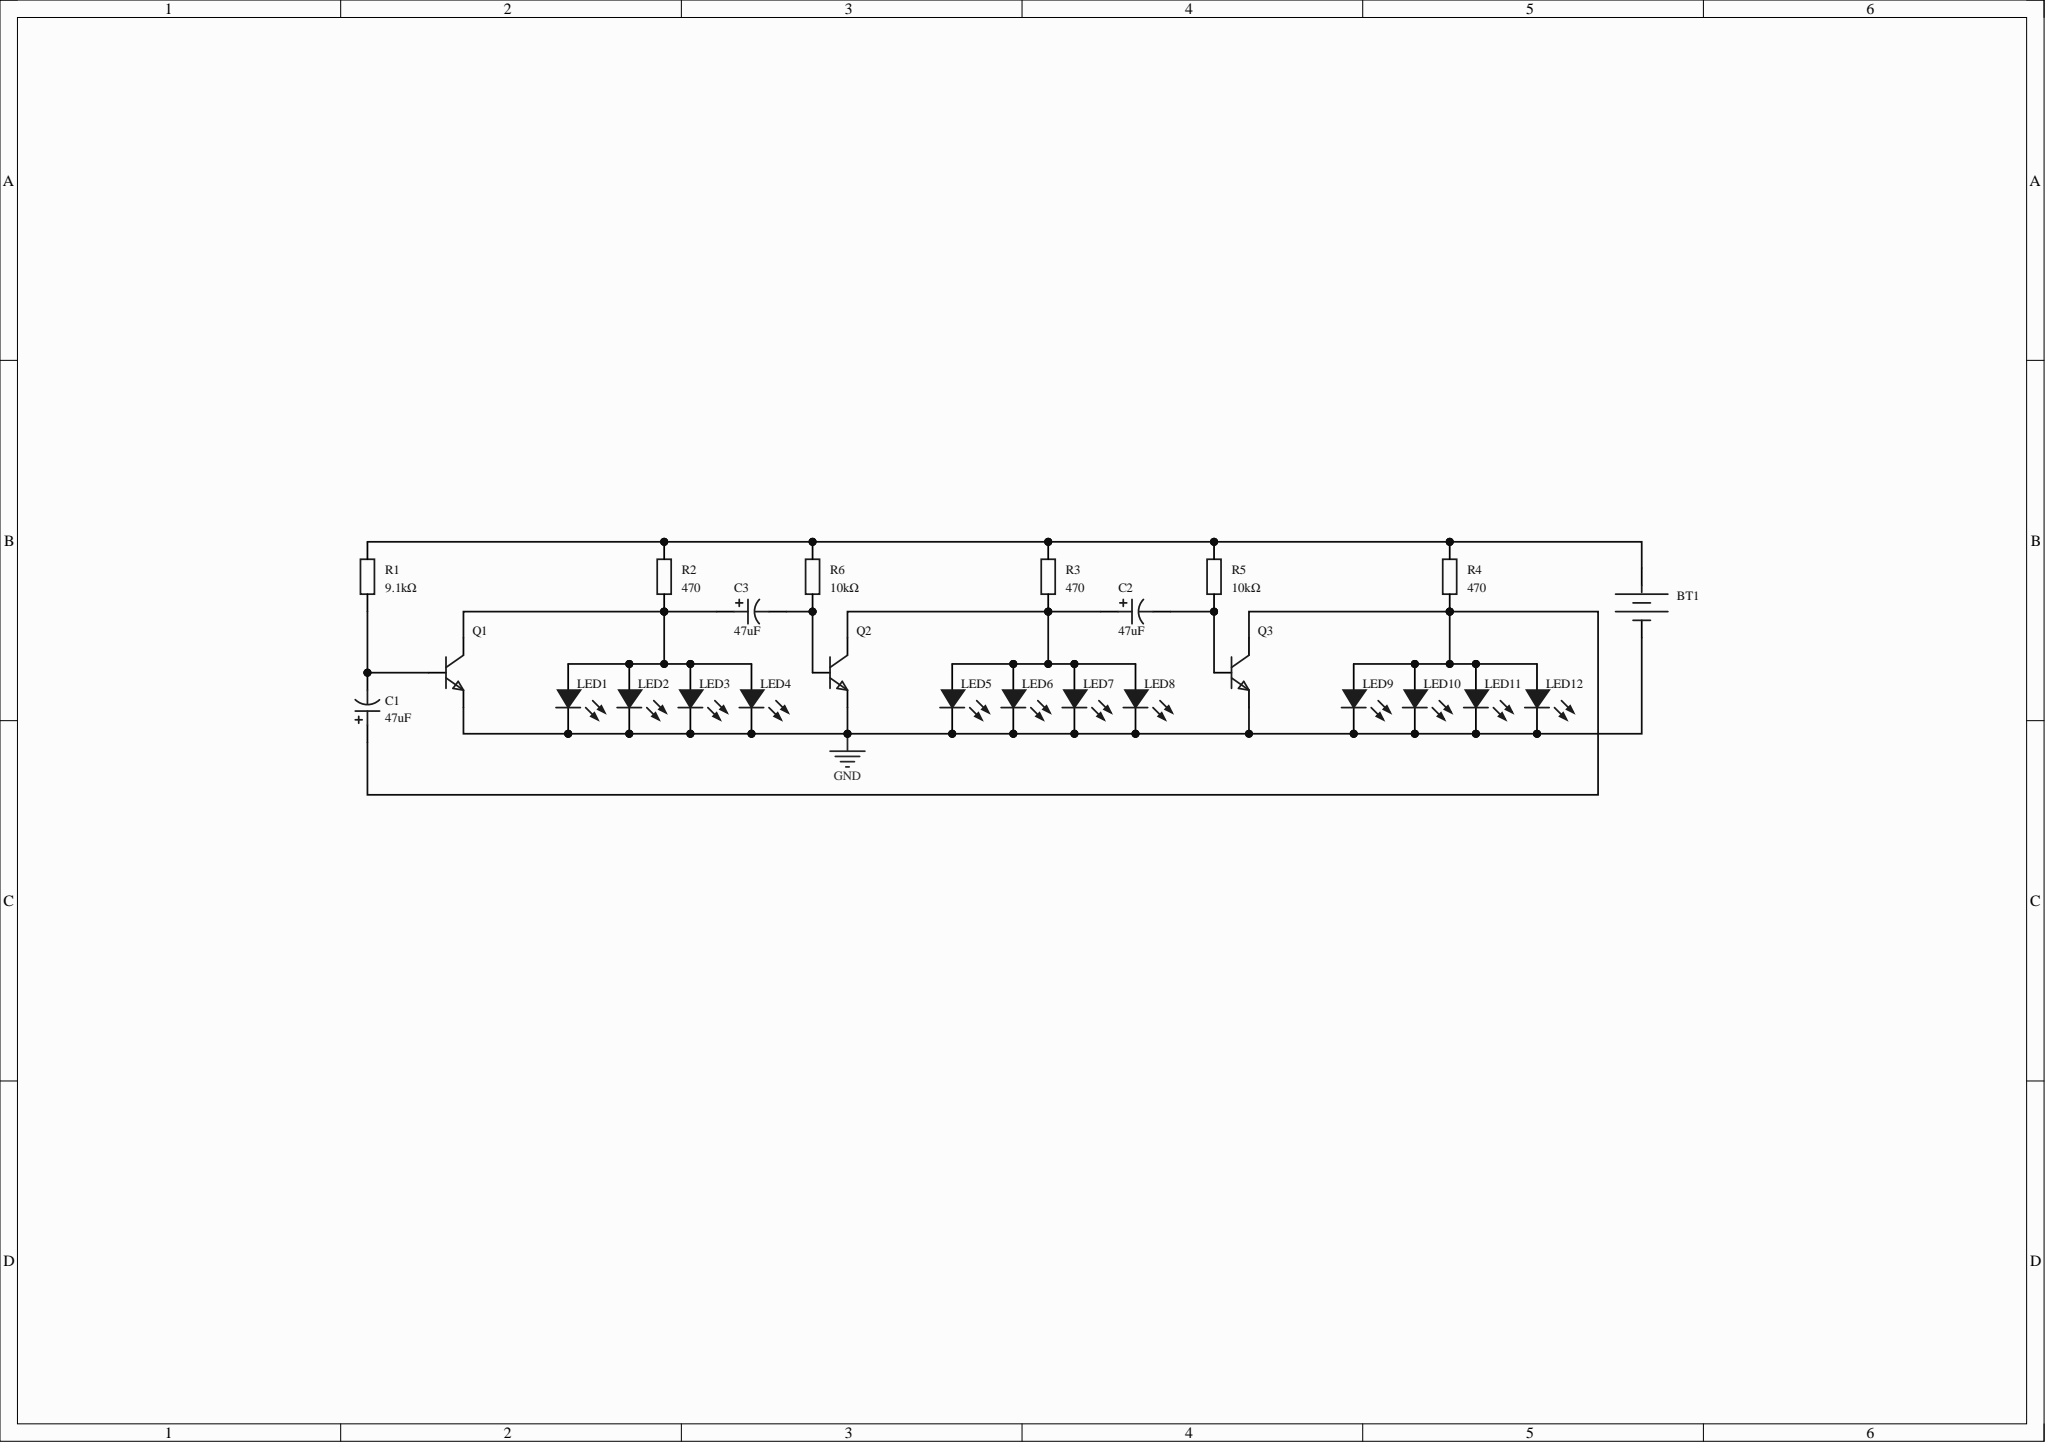Circuit board | Altium Designer | 25 parts | 8 nets
Bill of materials:
Comment,Description,Designator,Footprint,LibRef,Quantity
"9V battery wire clip Cu 100mm","","BT1","BAT-TH_2P-9VBATTERY","9V电池铜线扣 铜100mm","1"
"47uF","","C1, C2, C3","CAP-TH_BD6.3-P2.50-D0.5-FD","DHG016M476E110S1AA","3"
"","","LED1, LED2, LED3, LED4, LED5, LED6, LED7, LED8, LED9, LED10, LED11, LED12","LED-TH_5mm","LED_TH-B_5mm","12"
"","","Q1, Q2, Q3","S8050_TO_92","S8050_TO_NPN","3"
"9.1kΩ","","R1","Res_1/8W","Res_AXIAL-1/8W","1"
"470","","R2, R3, R4","Res_1/8W","Res_AXIAL-1/8W","3"
"10kΩ","","R5, R6","Res_1/8W","Res_AXIAL-1/8W","2"
Netlist (Protel format):
[
BT1
BAT-TH_2P-9VBATTERY
9V battery wire clip Cu 100mm



]
[
C1
CAP-TH_BD6.3-P2.50-D0.5-FD
47uF



]
[
C2
CAP-TH_BD6.3-P2.50-D0.5-FD
47uF



]
[
C3
CAP-TH_BD6.3-P2.50-D0.5-FD
47uF



]
[
LED1
LED-TH_5mm




]
[
LED2
LED-TH_5mm




]
[
LED3
LED-TH_5mm




]
[
LED4
LED-TH_5mm




]
[
LED5
LED-TH_5mm




]
[
LED6
LED-TH_5mm




]
[
LED7
LED-TH_5mm




]
[
LED8
LED-TH_5mm




]
[
LED9
LED-TH_5mm




]
[
LED10
LED-TH_5mm




]
[
LED11
LED-TH_5mm




]
[
LED12
LED-TH_5mm




]
[
Q1
S8050_TO_92




]
[
Q2
S8050_TO_92




]
[
Q3
S8050_TO_92




]
[
R1
Res_1/8W
9.1kΩ



]
[
R2
Res_1/8W
470



]
[
R3
Res_1/8W
470



]
[
R4
Res_1/8W
470



]
[
R5
Res_1/8W
10kΩ



]
[
R6
Res_1/8W
10kΩ



]
(
NetC3_2
C3-2
Q2-2
R6-1
)
(
NetC3_1
C3-1
LED1-1
LED2-1
LED3-1
LED4-1
Q1-3
R2-1
)
(
NetC2_2
C2-2
Q3-2
R5-1
)
(
NetC2_1
C2-1
LED5-1
LED6-1
LED7-1
LED8-1
Q2-3
R3-1
)
(
NetC1_2
C1-2
Q1-2
R1-1
)
(
NetC1_1
C1-1
LED9-1
LED10-1
LED11-1
LED12-1
Q3-3
R4-1
)
(
NetBT1_1
BT1-1
R1-2
R2-2
R3-2
R4-2
R5-2
R6-2
)
(
GND
BT1-2
LED1-2
LED2-2
LED3-2
LED4-2
LED5-2
LED6-2
LED7-2
LED8-2
LED9-2
LED10-2
LED11-2
LED12-2
Q1-1
Q2-1
Q3-1
)